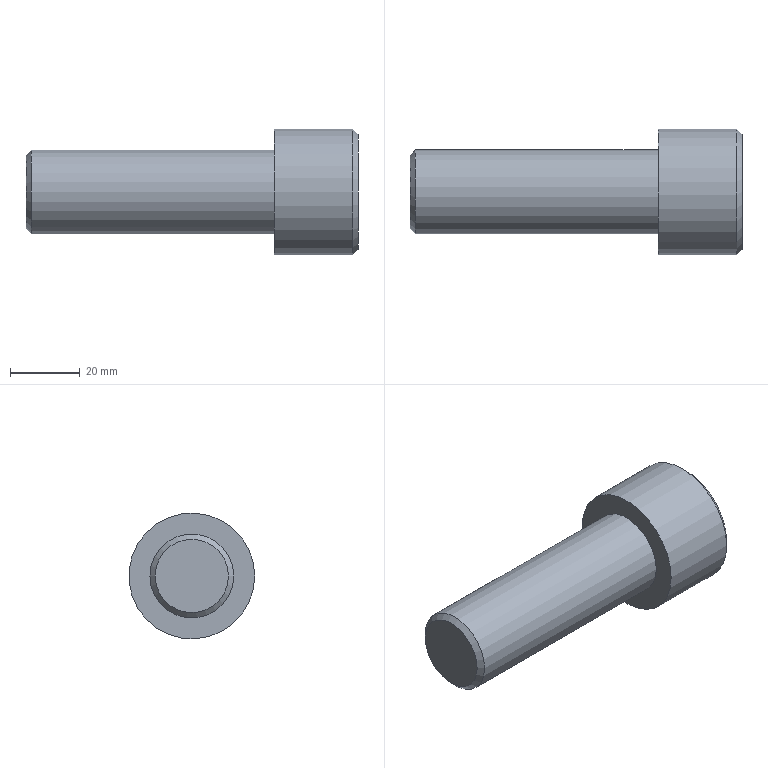Part | STEP file | solid 147 | 1 solid | 14 faces | box 95 x 36 x 36 mm | volume 52905 mm3 | plane 10 | cone 2 | cylinder 2 | commonest cylinder face diameters 24 x1 36 x1